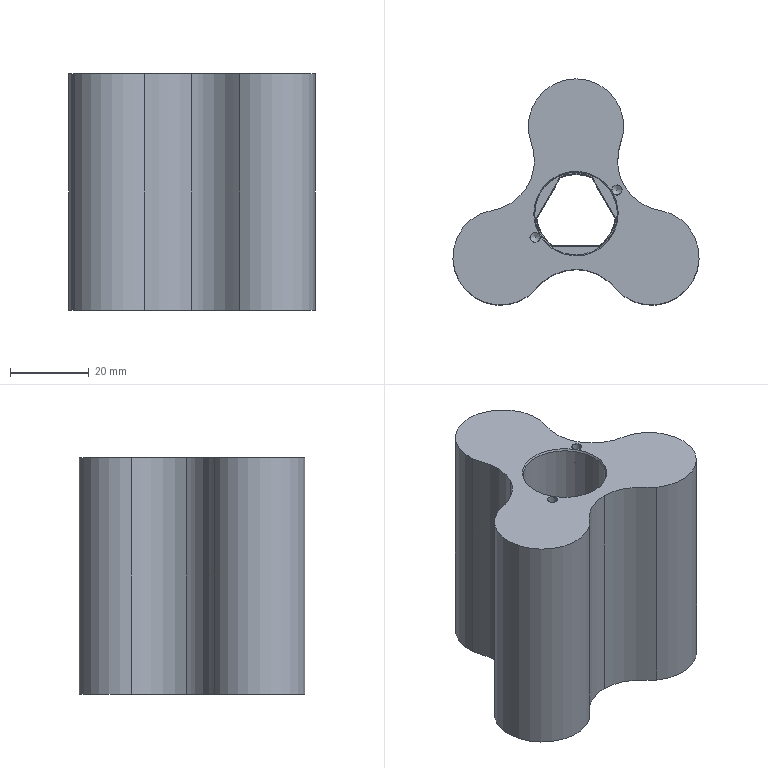NC program | NX | posted with a generic post | part box 62.563 x 57.43 x 60 mm
Lines 1 to 809 of 9902:
N10 G17 G21 G94 G90
(ZLEVEL_PROFILE , TOOL : D35R0.5)
N12 T05 M6
N14 G54
N16 G17 G0 G90 X34.081 Y14.702 S2000 M3
N18 G43 Z30. H5
N20 Z3.
N22 G94 G1 X34.768 Y14.292 Z2.979 F1000.
N24 X35.942 Y13.56 Z2.943
N26 X36.621 Y13.081 Z2.921
N28 X37.705 Y12.221 Z2.885
N30 X38.759 Y11.377 Z2.849
N32 X41.001 Y9.198 Z2.768
N34 X43.008 Y6.801 Z2.686
N36 X44.758 Y4.21 Z2.604
N38 X45.403 Y3.024 Z2.568
N40 X46.076 Y1.715 Z2.53
N42 X46.85 Y-0.079 Z2.479
N44 X47.34 Y-1.467 Z2.44
N46 X47.772 Y-2.754 Z2.405
N48 X48.413 Y-5.432 Z2.333
N50 X48.811 Y-8.158 Z2.26
N52 X48.887 Y-9.513 Z2.225
N54 X48.949 Y-10.934 Z2.188
N56 X48.926 Y-12.252 Z2.153
N58 X48.813 Y-13.67 Z2.116
N60 X48.67 Y-15.116 Z2.078
N62 X48.468 Y-16.38 Z2.044
N64 X48.155 Y-17.799 Z2.006
N66 X47.809 Y-19.216 Z1.968
N68 X47.485 Y-20.28 Z1.939
N70 X46.98 Y-21.648 Z1.901
N72 X46.461 Y-22.979 Z1.863
N74 X45.924 Y-24.141 Z1.83
N76 X45.247 Y-25.399 Z1.792
N78 X44.538 Y-26.658 Z1.755
N80 X43.83 Y-27.755 Z1.72
N82 X42.975 Y-28.92 Z1.683
N84 X42.111 Y-30.053 Z1.645
N86 X41.288 Y-31.006 Z1.612
N88 X40.293 Y-32.026 Z1.575
N90 X39.262 Y-33.044 Z1.537
N92 X38.381 Y-33.819 Z1.506
N94 X37.238 Y-34.71 Z1.468
N96 X36.081 Y-35.577 Z1.43
N98 X35.037 Y-36.266 Z1.398
N100 X33.785 Y-36.989 Z1.36
N102 X32.519 Y-37.687 Z1.322
N104 X31.363 Y-38.237 Z1.289
N106 X30.022 Y-38.778 Z1.251
N108 X28.669 Y-39.293 Z1.213
N110 X27.508 Y-39.657 Z1.181
N112 X26.103 Y-40.009 Z1.143
N114 X24.693 Y-40.333 Z1.105
N116 X23.473 Y-40.538 Z1.073
N118 X22.035 Y-40.692 Z1.035
N120 X20.686 Y-40.818 Z0.999
N122 X17.93 Y-40.829 Z0.927
N124 X15.183 Y-40.591 Z0.855
N126 X13.849 Y-40.355 Z0.819
N128 X12.439 Y-40.086 Z0.782
N130 X11.212 Y-39.775 Z0.749
N132 X9.844 Y-39.339 Z0.711
N134 X8.462 Y-38.866 Z0.673
N136 X7.29 Y-38.386 Z0.64
N138 X5.973 Y-37.755 Z0.601
N140 X4.673 Y-37.095 Z0.563
N142 X2.567 Y-35.817 Z0.499
N144 X1.381 Y-34.968 Z0.461
N146 X0. Y-33.831 Z0.414
N148 X-0.748 Y-34.477 Z0.388
N150 X-1.544 Y-35.061 Z0.362
N152 X-1.964 Y-35.371 Z0.348
N154 X-4.511 Y-36.983 Z0.269
N156 X-5.756 Y-37.671 Z0.232
N158 X-7.345 Y-38.413 Z0.186
N160 X-8.673 Y-38.925 Z0.149
N162 X-10.023 Y-39.419 Z0.111
N164 X-11.278 Y-39.793 Z0.077
N166 X-12.679 Y-40.119 Z0.039
N168 X-13.992 Y-40.409 Z0.004
N170 X-17.003 Y-40.78 Z-0.075
N172 X-20.037 Y-40.847 Z-0.155
N174 X-23.061 Y-40.609 Z-0.234
N176 X-26.047 Y-40.069 Z-0.314
N178 X-27.342 Y-39.705 Z-0.349
N180 G2 X-32.754 Y-37.545 R34.234 F2200.
N182 X-36.226 Y-35.451 R34.326
N184 X-39.523 Y-32.776 R34.837
N186 X-42.277 Y-29.815 R35.845
N188 X-44.661 Y-26.417 R34.925
N190 X-46.496 Y-22.842 R34.367
N192 X-47.873 Y-18.913 R34.46
N194 X-48.686 Y-14.846 R34.715
N196 X-48.925 Y-10.687 R34.596
N198 X-47.701 Y-2.6 R30.734
N200 X-46.246 Y1.29 R35.982
N202 X-44.291 Y4.897 R34.967
N204 X-38.981 Y11.153 R30.974
N206 X-35.728 Y13.674 R34.245
N208 X-32.188 Y15.709 R35.224
N210 X-29.299 Y16.914 R25.445
N212 X-29.651 Y19.398 R24.652
N214 G1 X-29.696 Y19.985
N216 X-29.762 Y22.921
N218 G2 X-29.371 Y26.989 R35.892
N220 X-26.892 Y34.896 R30.541
N222 X-22.351 Y41.786 R31.471
N224 X-19.415 Y44.69 R35.483
N226 X-12.506 Y49.138 R31.087
N228 X-8.729 Y50.583 R36.254
N230 X-4.678 Y51.521 R35.079
N232 X3.508 Y51.684 R30.536
N234 X7.601 Y50.904 R34.85
N236 X11.509 Y49.576 R36.085
N238 X18.574 Y45.387 R31.015
N240 X21.606 Y42.602 R35.518
N242 X26.376 Y35.929 R30.936
N244 X29.667 Y24.773 R30.369
N246 X29.696 Y19.985 R35.826
N248 X29.302 Y16.938 R24.197
N250 G1 X29.316 Y16.911
N252 X29.499 Y16.844
N254 G2 X32.233 Y15.681 R23.446
N256 X34.768 Y14.292 R40.155
N258 X37.705 Y12.221 R31.887
N260 X45.403 Y3.024 R30.367
N262 X47.34 Y-1.467 R36.082
N264 X48.887 Y-9.513 R30.683
N266 X48.813 Y-13.67 R33.705
N268 X48.155 Y-17.799 R35.18
N270 X46.98 Y-21.648 R35.42
N272 X45.247 Y-25.399 R33.989
N274 X42.975 Y-28.92 R34.793
N276 X40.293 Y-32.026 R33.805
N278 X37.238 Y-34.71 R34.994
N280 X33.785 Y-36.989 R34.837
N282 X30.022 Y-38.778 R34.827
N284 X26.103 Y-40.009 R34.934
N286 X22.035 Y-40.692 R34.846
N288 X13.849 Y-40.355 R30.565
N290 X9.844 Y-39.339 R34.343
N292 X5.973 Y-37.755 R35.502
N294 X1.381 Y-34.968 R35.404
N296 G1 X0. Y-33.831
N298 G2 X-1.544 Y-35.061 R24.993
N300 G1 X-1.964 Y-35.371
N302 X-4.511 Y-36.983
N304 G2 X-8.673 Y-38.925 R33.739
N306 X-12.679 Y-40.119 R34.443
N308 X-27.342 Y-39.705 R30.15
N310 G1 X-28.016 Y-39.471 Z-0.361
N312 X-28.698 Y-39.259 Z-0.374
N314 X-29.373 Y-39.026 Z-0.386
N316 X-30.04 Y-38.773 Z-0.399
N318 X-30.7 Y-38.5 Z-0.411
N320 X-31.355 Y-38.217 Z-0.424
N322 X-32.003 Y-37.917 Z-0.436
N324 X-32.644 Y-37.603 Z-0.449
N326 X-33.276 Y-37.272 Z-0.461
N328 X-33.901 Y-36.926 Z-0.473
N330 X-34.517 Y-36.565 Z-0.486
N332 X-35.125 Y-36.191 Z-0.498
N334 X-35.723 Y-35.8 Z-0.511
N336 X-36.311 Y-35.396 Z-0.523
N338 X-36.89 Y-34.978 Z-0.536
N340 X-37.458 Y-34.546 Z-0.548
N342 X-38.016 Y-34.1 Z-0.561
N344 X-38.563 Y-33.641 Z-0.573
N346 X-39.099 Y-33.169 Z-0.586
N348 X-39.623 Y-32.685 Z-0.598
N350 X-40.136 Y-32.188 Z-0.61
N352 X-40.637 Y-31.679 Z-0.623
N354 X-41.125 Y-31.158 Z-0.635
N356 X-41.6 Y-30.625 Z-0.648
N358 X-42.063 Y-30.082 Z-0.66
N360 X-42.513 Y-29.527 Z-0.673
N362 X-42.949 Y-28.961 Z-0.685
N364 X-43.371 Y-28.386 Z-0.698
N366 G2 X-31.616 Y15.985 R29.776
N368 X-29.307 Y16.858 R17.65
N370 X-29.651 Y19.386 R70.972
N372 X29.651 Y19.386 R-29.776
N374 X29.302 Y16.938 R25.206
N376 G1 X29.316 Y16.911
N378 X29.499 Y16.844
N380 G2 X31.585 Y15.999 R26.764
N382 X1.965 Y-35.372 R-29.776
N384 G1 X0.757 Y-34.464
N386 X0.606 Y-34.309
N388 X0.559 Y-34.3
N390 X0. Y-33.831
N392 G2 X-1.964 Y-35.371 R28.191
N394 X-27.337 Y-39.689 R29.776
N396 G1 X-28.021 Y-39.485 Z-0.71
N398 X-28.7 Y-39.264 Z-0.723
N400 X-29.373 Y-39.027 Z-0.735
N402 X-30.041 Y-38.774 Z-0.748
N404 X-30.702 Y-38.506 Z-0.76
N406 X-31.356 Y-38.221 Z-0.772
N408 X-32.004 Y-37.921 Z-0.785
N410 X-32.644 Y-37.605 Z-0.797
N412 X-33.276 Y-37.274 Z-0.81
N414 X-33.901 Y-36.928 Z-0.822
N416 X-34.516 Y-36.567 Z-0.835
N418 X-35.123 Y-36.192 Z-0.847
N420 X-35.721 Y-35.802 Z-0.86
N422 X-36.309 Y-35.398 Z-0.872
N424 X-36.888 Y-34.979 Z-0.885
N426 X-37.456 Y-34.548 Z-0.897
N428 X-38.014 Y-34.102 Z-0.909
N430 X-38.561 Y-33.644 Z-0.922
N432 X-39.096 Y-33.172 Z-0.934
N434 X-39.621 Y-32.688 Z-0.947
N436 X-40.133 Y-32.191 Z-0.959
N438 X-40.634 Y-31.682 Z-0.972
N440 X-41.122 Y-31.161 Z-0.984
N442 X-41.597 Y-30.629 Z-0.997
N444 X-42.06 Y-30.086 Z-1.009
N446 X-42.509 Y-29.531 Z-1.022
N448 X-42.945 Y-28.966 Z-1.034
N450 X-43.368 Y-28.391 Z-1.047
N452 G2 X-31.616 Y15.985 R29.776
N454 X-29.307 Y16.858 R17.65
N456 X-29.651 Y19.386 R70.933
N458 X29.651 Y19.386 R-29.776
N460 X29.302 Y16.938 R25.206
N462 G1 X29.316 Y16.911
N464 X29.499 Y16.844
N466 G2 X31.585 Y15.999 R26.764
N468 X1.965 Y-35.372 R-29.776
N470 G1 X0.757 Y-34.464
N472 X0.606 Y-34.309
N474 X0.559 Y-34.3
N476 X0. Y-33.831
N478 G2 X-1.964 Y-35.371 R28.19
N480 X-27.337 Y-39.689 R29.776
N482 G1 X-28.021 Y-39.485 Z-1.059
N484 X-28.7 Y-39.264 Z-1.071
N486 X-29.373 Y-39.027 Z-1.084
N488 X-30.041 Y-38.774 Z-1.096
N490 X-30.702 Y-38.506 Z-1.109
N492 X-31.356 Y-38.221 Z-1.121
N494 X-32.004 Y-37.921 Z-1.134
N496 X-32.644 Y-37.605 Z-1.146
N498 X-33.276 Y-37.274 Z-1.159
N500 X-33.901 Y-36.928 Z-1.171
N502 X-34.516 Y-36.567 Z-1.184
N504 X-35.123 Y-36.192 Z-1.196
N506 X-35.721 Y-35.802 Z-1.208
N508 X-36.309 Y-35.398 Z-1.221
N510 X-36.888 Y-34.979 Z-1.233
N512 X-37.456 Y-34.548 Z-1.246
N514 X-38.014 Y-34.102 Z-1.258
N516 X-38.561 Y-33.644 Z-1.271
N518 X-39.096 Y-33.172 Z-1.283
N520 X-39.621 Y-32.688 Z-1.296
N522 X-40.133 Y-32.191 Z-1.308
N524 X-40.634 Y-31.682 Z-1.321
N526 X-41.122 Y-31.161 Z-1.333
N528 X-41.597 Y-30.629 Z-1.346
N530 X-42.06 Y-30.086 Z-1.358
N532 X-42.509 Y-29.531 Z-1.37
N534 X-42.945 Y-28.966 Z-1.383
N536 X-43.368 Y-28.391 Z-1.395
N538 G2 X-31.616 Y15.985 R29.776
N540 X-29.307 Y16.858 R17.65
N542 X-29.651 Y19.386 R70.893
N544 X29.651 Y19.386 R-29.776
N546 X29.302 Y16.938 R25.205
N548 G1 X29.316 Y16.911
N550 X29.499 Y16.844
N552 G2 X31.585 Y15.999 R26.763
N554 X1.965 Y-35.372 R-29.776
N556 G1 X0.757 Y-34.464
N558 X0.606 Y-34.309
N560 X0.559 Y-34.3
N562 X0. Y-33.831
N564 G2 X-1.964 Y-35.371 R28.188
N566 X-27.337 Y-39.689 R29.776
N568 G1 X-28.021 Y-39.485 Z-1.408
N570 X-28.7 Y-39.264 Z-1.42
N572 X-29.373 Y-39.027 Z-1.433
N574 X-30.041 Y-38.774 Z-1.445
N576 X-30.702 Y-38.506 Z-1.458
N578 X-31.356 Y-38.221 Z-1.47
N580 X-32.004 Y-37.921 Z-1.483
N582 X-32.644 Y-37.605 Z-1.495
N584 X-33.276 Y-37.274 Z-1.507
N586 X-33.901 Y-36.928 Z-1.52
N588 X-34.516 Y-36.567 Z-1.532
N590 X-35.123 Y-36.192 Z-1.545
N592 X-35.721 Y-35.802 Z-1.557
N594 X-36.309 Y-35.398 Z-1.57
N596 X-36.888 Y-34.979 Z-1.582
N598 X-37.456 Y-34.548 Z-1.595
N600 X-38.014 Y-34.102 Z-1.607
N602 X-38.561 Y-33.644 Z-1.62
N604 X-39.096 Y-33.172 Z-1.632
N606 X-39.621 Y-32.688 Z-1.645
N608 X-40.133 Y-32.191 Z-1.657
N610 X-40.634 Y-31.682 Z-1.669
N612 X-41.122 Y-31.161 Z-1.682
N614 X-41.597 Y-30.629 Z-1.694
N616 X-42.06 Y-30.086 Z-1.707
N618 X-42.509 Y-29.531 Z-1.719
N620 X-42.945 Y-28.966 Z-1.732
N622 X-43.368 Y-28.391 Z-1.744
N624 G2 X-31.616 Y15.985 R29.776
N626 X-29.307 Y16.858 R17.65
N628 X-29.651 Y19.386 R70.854
N630 X29.651 Y19.386 R-29.776
N632 X29.302 Y16.938 R25.204
N634 G1 X29.316 Y16.911
N636 X29.499 Y16.844
N638 G2 X31.585 Y15.999 R26.763
N640 X1.965 Y-35.372 R-29.776
N642 G1 X0.757 Y-34.464
N644 X0.606 Y-34.309
N646 X0.559 Y-34.3
N648 X0. Y-33.831
N650 G2 X-1.964 Y-35.371 R28.187
N652 X-27.337 Y-39.689 R29.776
N654 G1 X-28.021 Y-39.485 Z-1.757
N656 X-28.7 Y-39.264 Z-1.769
N658 X-29.373 Y-39.027 Z-1.782
N660 X-30.041 Y-38.774 Z-1.794
N662 X-30.702 Y-38.506 Z-1.806
N664 X-31.356 Y-38.221 Z-1.819
N666 X-32.004 Y-37.921 Z-1.831
N668 X-32.644 Y-37.605 Z-1.844
N670 X-33.276 Y-37.274 Z-1.856
N672 X-33.901 Y-36.928 Z-1.869
N674 X-34.516 Y-36.567 Z-1.881
N676 X-35.123 Y-36.192 Z-1.894
N678 X-35.721 Y-35.802 Z-1.906
N680 X-36.309 Y-35.398 Z-1.919
N682 X-36.888 Y-34.979 Z-1.931
N684 X-37.456 Y-34.548 Z-1.944
N686 X-38.014 Y-34.102 Z-1.956
N688 X-38.561 Y-33.644 Z-1.968
N690 X-39.096 Y-33.172 Z-1.981
N692 X-39.621 Y-32.688 Z-1.993
N694 X-40.133 Y-32.191 Z-2.006
N696 X-40.634 Y-31.682 Z-2.018
N698 X-41.122 Y-31.161 Z-2.031
N700 X-41.597 Y-30.629 Z-2.043
N702 X-42.06 Y-30.086 Z-2.056
N704 X-42.509 Y-29.531 Z-2.068
N706 X-42.945 Y-28.966 Z-2.081
N708 X-43.368 Y-28.391 Z-2.093
N710 G2 X-31.616 Y15.985 R29.776
N712 X-29.307 Y16.858 R17.65
N714 X-29.651 Y19.386 R70.814
N716 X29.651 Y19.386 R-29.776
N718 X29.302 Y16.938 R25.203
N720 G1 X29.316 Y16.911
N722 X29.499 Y16.844
N724 G2 X31.585 Y15.999 R26.762
N726 X1.965 Y-35.372 R-29.776
N728 G1 X0.757 Y-34.464
N730 X0.606 Y-34.309
N732 X0.559 Y-34.3
N734 X0. Y-33.831
N736 G2 X-1.964 Y-35.371 R28.186
N738 X-27.337 Y-39.689 R29.776
N740 G1 X-28.021 Y-39.485 Z-2.105
N742 X-28.7 Y-39.264 Z-2.118
N744 X-29.373 Y-39.027 Z-2.13
N746 X-30.041 Y-38.774 Z-2.143
N748 X-30.702 Y-38.506 Z-2.155
N750 X-31.356 Y-38.221 Z-2.168
N752 X-32.004 Y-37.921 Z-2.18
N754 X-32.644 Y-37.605 Z-2.193
N756 X-33.276 Y-37.274 Z-2.205
N758 X-33.901 Y-36.928 Z-2.218
N760 X-34.516 Y-36.567 Z-2.23
N762 X-35.123 Y-36.192 Z-2.243
N764 X-35.721 Y-35.802 Z-2.255
N766 X-36.309 Y-35.398 Z-2.267
N768 X-36.888 Y-34.979 Z-2.28
N770 X-37.456 Y-34.548 Z-2.292
N772 X-38.014 Y-34.102 Z-2.305
N774 X-38.561 Y-33.644 Z-2.317
N776 X-39.096 Y-33.172 Z-2.33
N778 X-39.621 Y-32.688 Z-2.342
N780 X-40.133 Y-32.191 Z-2.355
N782 X-40.634 Y-31.682 Z-2.367
N784 X-41.122 Y-31.161 Z-2.38
N786 X-41.597 Y-30.629 Z-2.392
N788 X-42.06 Y-30.086 Z-2.404
N790 X-42.509 Y-29.531 Z-2.417
N792 X-42.945 Y-28.966 Z-2.429
N794 X-43.368 Y-28.391 Z-2.442
N796 G2 X-31.616 Y15.985 R29.776
N798 X-29.307 Y16.858 R17.65
N800 X-29.651 Y19.386 R70.775
N802 X29.651 Y19.386 R-29.776
N804 X29.302 Y16.938 R25.203
N806 G1 X29.316 Y16.911
N808 X29.499 Y16.844
N810 G2 X31.585 Y15.999 R26.762
N812 X1.965 Y-35.372 R-29.776
N814 G1 X0.757 Y-34.464
N816 X0.606 Y-34.309
N818 X0.559 Y-34.3
N820 X0. Y-33.831
N822 G2 X-1.964 Y-35.371 R28.185
N824 X-27.337 Y-39.689 R29.776
N826 G1 X-28.021 Y-39.485 Z-2.454
N828 X-28.7 Y-39.264 Z-2.467
N830 X-29.373 Y-39.027 Z-2.479
N832 X-30.041 Y-38.774 Z-2.492
N834 X-30.702 Y-38.506 Z-2.504
N836 X-31.356 Y-38.221 Z-2.517
N838 X-32.004 Y-37.921 Z-2.529
N840 X-32.644 Y-37.605 Z-2.542
N842 X-33.276 Y-37.274 Z-2.554
N844 X-33.901 Y-36.928 Z-2.566
N846 X-34.516 Y-36.567 Z-2.579
N848 X-35.123 Y-36.192 Z-2.591
N850 X-35.721 Y-35.802 Z-2.604
N852 X-36.309 Y-35.398 Z-2.616
N854 X-36.888 Y-34.979 Z-2.629
N856 X-37.456 Y-34.548 Z-2.641
N858 X-38.014 Y-34.102 Z-2.654
N860 X-38.561 Y-33.644 Z-2.666
N862 X-39.096 Y-33.172 Z-2.679
N864 X-39.621 Y-32.688 Z-2.691
N866 X-40.133 Y-32.191 Z-2.703
N868 X-40.634 Y-31.682 Z-2.716
N870 X-41.122 Y-31.161 Z-2.728
N872 X-41.597 Y-30.629 Z-2.741
N874 X-42.06 Y-30.086 Z-2.753
N876 X-42.509 Y-29.531 Z-2.766
N878 X-42.945 Y-28.966 Z-2.778
N880 X-43.368 Y-28.391 Z-2.791
N882 G2 X-31.616 Y15.985 R29.776
N884 X-29.307 Y16.858 R17.65
N886 X-29.651 Y19.386 R70.736
N888 X29.651 Y19.386 R-29.776
N890 X29.302 Y16.938 R25.202
N892 G1 X29.316 Y16.911
N894 X29.499 Y16.844
N896 G2 X31.585 Y15.999 R26.762
N898 X1.965 Y-35.372 R-29.776
N900 G1 X0.757 Y-34.464
N902 X0.606 Y-34.309
N904 X0.559 Y-34.3
N906 X0. Y-33.831
N908 G2 X-1.964 Y-35.371 R28.183
N910 X-27.337 Y-39.689 R29.776
N912 G1 X-28.021 Y-39.485 Z-2.803
N914 X-28.7 Y-39.264 Z-2.816
N916 X-29.373 Y-39.027 Z-2.828
N918 X-30.041 Y-38.774 Z-2.841
N920 X-30.702 Y-38.506 Z-2.853
N922 X-31.356 Y-38.221 Z-2.865
N924 X-32.004 Y-37.921 Z-2.878
N926 X-32.644 Y-37.605 Z-2.89
N928 X-33.276 Y-37.274 Z-2.903
N930 X-33.901 Y-36.928 Z-2.915
N932 X-34.516 Y-36.567 Z-2.928
N934 X-35.123 Y-36.192 Z-2.94
N936 X-35.721 Y-35.802 Z-2.953
N938 X-36.309 Y-35.398 Z-2.965
N940 X-36.888 Y-34.979 Z-2.978
N942 X-37.456 Y-34.548 Z-2.99
N944 X-38.014 Y-34.102 Z-3.002
N946 X-38.561 Y-33.644 Z-3.015
N948 X-39.096 Y-33.172 Z-3.027
N950 X-39.621 Y-32.688 Z-3.04
N952 X-40.133 Y-32.191 Z-3.052
N954 X-40.634 Y-31.682 Z-3.065
N956 X-41.122 Y-31.161 Z-3.077
N958 X-41.597 Y-30.629 Z-3.09
N960 X-42.06 Y-30.086 Z-3.102
N962 X-42.509 Y-29.531 Z-3.115
N964 X-42.945 Y-28.966 Z-3.127
N966 X-43.368 Y-28.391 Z-3.14
N968 G2 X-31.616 Y15.985 R29.776
N970 X-29.307 Y16.858 R17.65
N972 X-29.651 Y19.386 R70.696
N974 X29.651 Y19.386 R-29.776
N976 X29.302 Y16.938 R25.201
N978 G1 X29.316 Y16.911
N980 X29.499 Y16.844
N982 G2 X31.585 Y15.999 R26.761
N984 X1.965 Y-35.372 R-29.776
N986 G1 X0.757 Y-34.464
N988 X0.606 Y-34.309
N990 X0.559 Y-34.3
N992 X0. Y-33.831
N994 G2 X-1.964 Y-35.371 R28.182
N996 X-27.337 Y-39.689 R29.776
N998 G1 X-28.021 Y-39.485 Z-3.152
N1000 X-28.7 Y-39.264 Z-3.164
N1002 X-29.373 Y-39.027 Z-3.177
N1004 X-30.041 Y-38.774 Z-3.189
N1006 X-30.702 Y-38.506 Z-3.202
N1008 X-31.356 Y-38.221 Z-3.214
N1010 X-32.004 Y-37.921 Z-3.227
N1012 X-32.644 Y-37.605 Z-3.239
N1014 X-33.276 Y-37.274 Z-3.252
N1016 X-33.901 Y-36.928 Z-3.264
N1018 X-34.516 Y-36.567 Z-3.277
N1020 X-35.123 Y-36.192 Z-3.289
N1022 X-35.721 Y-35.802 Z-3.301
N1024 X-36.309 Y-35.398 Z-3.314
N1026 X-36.888 Y-34.979 Z-3.326
N1028 X-37.456 Y-34.548 Z-3.339
N1030 X-38.014 Y-34.102 Z-3.351
N1032 X-38.561 Y-33.644 Z-3.364
N1034 X-39.096 Y-33.172 Z-3.376
N1036 X-39.621 Y-32.688 Z-3.389
N1038 X-40.133 Y-32.191 Z-3.401
N1040 X-40.634 Y-31.682 Z-3.414
N1042 X-41.122 Y-31.161 Z-3.426
N1044 X-41.597 Y-30.629 Z-3.439
N1046 X-42.06 Y-30.086 Z-3.451
N1048 X-42.509 Y-29.531 Z-3.463
N1050 X-42.945 Y-28.966 Z-3.476
N1052 X-43.368 Y-28.391 Z-3.488
N1054 G2 X-31.616 Y15.985 R29.776
N1056 X-29.307 Y16.858 R17.65
N1058 X-29.651 Y19.386 R70.657
N1060 X29.651 Y19.386 R-29.776
N1062 X29.302 Y16.938 R25.2
N1064 G1 X29.316 Y16.911
N1066 X29.499 Y16.844
N1068 G2 X31.585 Y15.999 R26.761
N1070 X1.965 Y-35.372 R-29.776
N1072 G1 X0.757 Y-34.464
N1074 X0.606 Y-34.309
N1076 X0.559 Y-34.3
N1078 X0. Y-33.831
N1080 G2 X-1.964 Y-35.371 R28.181
N1082 X-27.337 Y-39.689 R29.776
N1084 G1 X-28.021 Y-39.485 Z-3.501
N1086 X-28.7 Y-39.264 Z-3.513
N1088 X-29.373 Y-39.027 Z-3.526
N1090 X-30.041 Y-38.774 Z-3.538
N1092 X-30.702 Y-38.506 Z-3.551
N1094 X-31.356 Y-38.221 Z-3.563
N1096 X-32.004 Y-37.921 Z-3.576
N1098 X-32.644 Y-37.605 Z-3.588
N1100 X-33.276 Y-37.274 Z-3.6
N1102 X-33.901 Y-36.928 Z-3.613
N1104 X-34.516 Y-36.567 Z-3.625
N1106 X-35.123 Y-36.192 Z-3.638
N1108 X-35.721 Y-35.802 Z-3.65
N1110 X-36.309 Y-35.398 Z-3.663
N1112 X-36.888 Y-34.979 Z-3.675
N1114 X-37.456 Y-34.548 Z-3.688
N1116 X-38.014 Y-34.102 Z-3.7
N1118 X-38.561 Y-33.644 Z-3.713
N1120 X-39.096 Y-33.172 Z-3.725
N1122 X-39.621 Y-32.688 Z-3.738
N1124 X-40.133 Y-32.191 Z-3.75
N1126 X-40.634 Y-31.682 Z-3.762
N1128 X-41.122 Y-31.161 Z-3.775
N1130 X-41.597 Y-30.629 Z-3.787
N1132 X-42.06 Y-30.086 Z-3.8
N1134 X-42.509 Y-29.531 Z-3.812
N1136 X-42.945 Y-28.966 Z-3.825
N1138 X-43.368 Y-28.391 Z-3.837
N1140 G2 X-31.616 Y15.985 R29.776
N1142 X-29.307 Y16.858 R17.65
N1144 X-29.651 Y19.386 R70.618
N1146 X29.651 Y19.386 R-29.776
N1148 X29.302 Y16.938 R25.2
N1150 G1 X29.316 Y16.911
N1152 X29.499 Y16.844
N1154 G2 X31.585 Y15.999 R26.76
N1156 X1.965 Y-35.372 R-29.776
N1158 G1 X0.757 Y-34.464
N1160 X0.606 Y-34.309
N1162 X0.559 Y-34.3
N1164 X0. Y-33.831
N1166 G2 X-1.964 Y-35.371 R28.18
N1168 X-27.337 Y-39.689 R29.776
N1170 G1 X-28.021 Y-39.485 Z-3.85
N1172 X-28.7 Y-39.264 Z-3.862
N1174 X-29.373 Y-39.027 Z-3.875
N1176 X-30.041 Y-38.774 Z-3.887
N1178 X-30.702 Y-38.506 Z-3.9
N1180 X-31.356 Y-38.221 Z-3.912
N1182 X-32.004 Y-37.921 Z-3.924
N1184 X-32.644 Y-37.605 Z-3.937
N1186 X-33.276 Y-37.274 Z-3.949
N1188 X-33.901 Y-36.928 Z-3.962
N1190 X-34.516 Y-36.567 Z-3.974
N1192 X-35.123 Y-36.192 Z-3.987
N1194 X-35.721 Y-35.802 Z-3.999
N1196 X-36.309 Y-35.398 Z-4.012
N1198 X-36.888 Y-34.979 Z-4.024
N1200 X-37.456 Y-34.548 Z-4.037
N1202 X-38.014 Y-34.102 Z-4.049
N1204 X-38.561 Y-33.644 Z-4.061
N1206 X-39.096 Y-33.172 Z-4.074
N1208 X-39.621 Y-32.688 Z-4.086
N1210 X-40.133 Y-32.191 Z-4.099
N1212 X-40.634 Y-31.682 Z-4.111
N1214 X-41.122 Y-31.161 Z-4.124
N1216 X-41.597 Y-30.629 Z-4.136
N1218 X-42.06 Y-30.086 Z-4.149
N1220 X-42.509 Y-29.531 Z-4.161
N1222 X-42.945 Y-28.966 Z-4.174
N1224 X-43.368 Y-28.391 Z-4.186
N1226 G2 X-31.616 Y15.985 R29.776
N1228 X-29.307 Y16.858 R17.65
N1230 X-29.651 Y19.386 R70.579
N1232 X29.651 Y19.386 R-29.776
N1234 X29.302 Y16.938 R25.199
N1236 G1 X29.316 Y16.911
N1238 X29.499 Y16.844
N1240 G2 X31.585 Y15.999 R26.76
N1242 X1.965 Y-35.372 R-29.776
N1244 G1 X0.757 Y-34.464
N1246 X0.606 Y-34.309
N1248 X0.559 Y-34.3
N1250 X0. Y-33.831
N1252 G2 X-1.964 Y-35.371 R28.178
N1254 X-27.337 Y-39.689 R29.776
N1256 G1 X-28.021 Y-39.485 Z-4.199
N1258 X-28.7 Y-39.264 Z-4.211
N1260 X-29.373 Y-39.027 Z-4.223
N1262 X-30.041 Y-38.774 Z-4.236
N1264 X-30.702 Y-38.506 Z-4.248
N1266 X-31.356 Y-38.221 Z-4.261
N1268 X-32.004 Y-37.921 Z-4.273
N1270 X-32.644 Y-37.605 Z-4.286
N1272 X-33.276 Y-37.274 Z-4.298
N1274 X-33.901 Y-36.928 Z-4.311
N1276 X-34.516 Y-36.567 Z-4.323
N1278 X-35.123 Y-36.192 Z-4.336
N1280 X-35.721 Y-35.802 Z-4.348
N1282 X-36.309 Y-35.398 Z-4.36
N1284 X-36.888 Y-34.979 Z-4.373
N1286 X-37.456 Y-34.548 Z-4.385
N1288 X-38.014 Y-34.102 Z-4.398
N1290 X-38.561 Y-33.644 Z-4.41
N1292 X-39.096 Y-33.172 Z-4.423
N1294 X-39.621 Y-32.688 Z-4.435
N1296 X-40.133 Y-32.191 Z-4.448
N1298 X-40.634 Y-31.682 Z-4.46
N1300 X-41.122 Y-31.161 Z-4.473
N1302 X-41.597 Y-30.629 Z-4.485
N1304 X-42.06 Y-30.086 Z-4.498
N1306 X-42.509 Y-29.531 Z-4.51
N1308 X-42.945 Y-28.966 Z-4.522
N1310 X-43.368 Y-28.391 Z-4.535
N1312 G2 X-31.616 Y15.985 R29.776
N1314 X-29.307 Y16.858 R17.65
N1316 X-29.651 Y19.386 R70.54
N1318 X29.651 Y19.386 R-29.776
N1320 X29.302 Y16.938 R25.198
N1322 G1 X29.316 Y16.911
N1324 X29.499 Y16.844
N1326 G2 X31.585 Y15.999 R26.759
N1328 X1.965 Y-35.372 R-29.776
N1330 G1 X0.757 Y-34.464
N1332 X0.606 Y-34.309
N1334 X0.559 Y-34.3
N1336 X0. Y-33.831
N1338 G2 X-1.964 Y-35.371 R28.177
N1340 X-27.337 Y-39.689 R29.776
N1342 G1 X-28.021 Y-39.485 Z-4.547
N1344 X-28.7 Y-39.264 Z-4.56
N1346 X-29.373 Y-39.027 Z-4.572
N1348 X-30.041 Y-38.774 Z-4.585
N1350 X-30.702 Y-38.506 Z-4.597
N1352 X-31.356 Y-38.221 Z-4.61
N1354 X-32.004 Y-37.921 Z-4.622
N1356 X-32.644 Y-37.605 Z-4.635
N1358 X-33.276 Y-37.274 Z-4.647
N1360 X-33.901 Y-36.928 Z-4.659
N1362 X-34.516 Y-36.567 Z-4.672
N1364 X-35.123 Y-36.192 Z-4.684
N1366 X-35.721 Y-35.802 Z-4.697
N1368 X-36.309 Y-35.398 Z-4.709
N1370 X-36.888 Y-34.979 Z-4.722
N1372 X-37.456 Y-34.548 Z-4.734
N1374 X-38.014 Y-34.102 Z-4.747
N1376 X-38.561 Y-33.644 Z-4.759
N1378 X-39.096 Y-33.172 Z-4.772
N1380 X-39.621 Y-32.688 Z-4.784
N1382 X-40.133 Y-32.191 Z-4.797
N1384 X-40.634 Y-31.682 Z-4.809
N1386 X-41.122 Y-31.161 Z-4.821
N1388 X-41.597 Y-30.629 Z-4.834
N1390 X-42.06 Y-30.086 Z-4.846
N1392 X-42.509 Y-29.531 Z-4.859
N1394 X-42.945 Y-28.966 Z-4.871
N1396 X-43.368 Y-28.391 Z-4.884
N1398 G2 X-31.616 Y15.985 R29.776
N1400 X-29.307 Y16.858 R17.65
N1402 X-29.651 Y19.386 R70.501
N1404 X29.651 Y19.386 R-29.776
N1406 X29.302 Y16.938 R25.197
N1408 G1 X29.316 Y16.911
N1410 X29.499 Y16.844
N1412 G2 X31.585 Y15.999 R26.759
N1414 X1.965 Y-35.372 R-29.776
N1416 G1 X0.757 Y-34.464
N1418 X0.606 Y-34.309
N1420 X0.559 Y-34.3
N1422 X0. Y-33.831
N1424 G2 X-1.964 Y-35.371 R28.176
N1426 X-27.337 Y-39.689 R29.776
N1428 G1 X-28.021 Y-39.485 Z-4.896
N1430 X-28.7 Y-39.264 Z-4.909
N1432 X-29.373 Y-39.027 Z-4.921
N1434 X-30.041 Y-38.774 Z-4.934
N1436 X-30.702 Y-38.506 Z-4.946
N1438 X-31.356 Y-38.221 Z-4.958
N1440 X-32.004 Y-37.921 Z-4.971
N1442 X-32.644 Y-37.605 Z-4.983
N1444 X-33.276 Y-37.274 Z-4.996
N1446 X-33.901 Y-36.928 Z-5.008
N1448 X-34.516 Y-36.567 Z-5.021
N1450 X-35.123 Y-36.192 Z-5.033
N1452 X-35.721 Y-35.802 Z-5.046
N1454 X-36.309 Y-35.398 Z-5.058
N1456 X-36.888 Y-34.979 Z-5.071
N1458 X-37.456 Y-34.548 Z-5.083
N1460 X-38.014 Y-34.102 Z-5.096
N1462 X-38.561 Y-33.644 Z-5.108
N1464 X-39.096 Y-33.172 Z-5.12
N1466 X-39.621 Y-32.688 Z-5.133
N1468 X-40.133 Y-32.191 Z-5.145
N1470 X-40.634 Y-31.682 Z-5.158
N1472 X-41.122 Y-31.161 Z-5.17
N1474 X-41.597 Y-30.629 Z-5.183
N1476 X-42.06 Y-30.086 Z-5.195
N1478 X-42.509 Y-29.531 Z-5.208
N1480 X-42.945 Y-28.966 Z-5.22
N1482 X-43.368 Y-28.391 Z-5.233
N1484 G2 X-31.616 Y15.985 R29.776
N1486 X-29.307 Y16.858 R17.65
N1488 X-29.651 Y19.386 R70.462
N1490 X29.651 Y19.386 R-29.776
N1492 X29.302 Y16.938 R25.197
N1494 G1 X29.316 Y16.911
N1496 X29.499 Y16.844
N1498 G2 X31.585 Y15.999 R26.759
N1500 X1.965 Y-35.372 R-29.776
N1502 G1 X0.757 Y-34.464
N1504 X0.606 Y-34.309
N1506 X0.559 Y-34.3
N1508 X0. Y-33.831
N1510 G2 X-1.964 Y-35.371 R28.174
N1512 X-27.337 Y-39.689 R29.776
N1514 G1 X-28.021 Y-39.485 Z-5.245
N1516 X-28.7 Y-39.264 Z-5.257
N1518 X-29.373 Y-39.027 Z-5.27
N1520 X-30.041 Y-38.774 Z-5.282
N1522 X-30.702 Y-38.506 Z-5.295
N1524 X-31.356 Y-38.221 Z-5.307
N1526 X-32.004 Y-37.921 Z-5.32
N1528 X-32.644 Y-37.605 Z-5.332
N1530 X-33.276 Y-37.274 Z-5.345
N1532 X-33.901 Y-36.928 Z-5.357
N1534 X-34.516 Y-36.567 Z-5.37
N1536 X-35.123 Y-36.192 Z-5.382
N1538 X-35.721 Y-35.802 Z-5.395
N1540 X-36.309 Y-35.398 Z-5.407
N1542 X-36.888 Y-34.979 Z-5.419
N1544 X-37.456 Y-34.548 Z-5.432
N1546 X-38.014 Y-34.102 Z-5.444
N1548 X-38.561 Y-33.644 Z-5.457
N1550 X-39.096 Y-33.172 Z-5.469
N1552 X-39.621 Y-32.688 Z-5.482
N1554 X-40.133 Y-32.191 Z-5.494
N1556 X-40.634 Y-31.682 Z-5.507
N1558 X-41.122 Y-31.161 Z-5.519
N1560 X-41.597 Y-30.629 Z-5.532
N1562 X-42.06 Y-30.086 Z-5.544
N1564 X-42.509 Y-29.531 Z-5.556
N1566 X-42.945 Y-28.966 Z-5.569
N1568 X-43.368 Y-28.391 Z-5.581
N1570 G2 X-31.616 Y15.985 R29.776
N1572 X-29.307 Y16.858 R17.65
N1574 X-29.651 Y19.386 R70.423
N1576 X29.651 Y19.386 R-29.776
N1578 X29.302 Y16.938 R25.196
N1580 G1 X29.316 Y16.911
N1582 X29.499 Y16.844
N1584 G2 X31.585 Y15.999 R26.758
N1586 X1.965 Y-35.372 R-29.776
N1588 G1 X0.757 Y-34.464
N1590 X0.606 Y-34.309
N1592 X0.559 Y-34.3
N1594 X0. Y-33.831
N1596 G2 X-1.964 Y-35.371 R28.173
N1598 X-27.337 Y-39.689 R29.776
N1600 G1 X-28.021 Y-39.485 Z-5.594
N1602 X-28.7 Y-39.264 Z-5.606
N1604 X-29.373 Y-39.027 Z-5.619
N1606 X-30.041 Y-38.774 Z-5.631
N1608 X-30.702 Y-38.506 Z-5.644
N1610 X-31.356 Y-38.221 Z-5.656
N1612 X-32.004 Y-37.921 Z-5.669
N1614 X-32.644 Y-37.605 Z-5.681
N1616 X-33.276 Y-37.274 Z-5.694